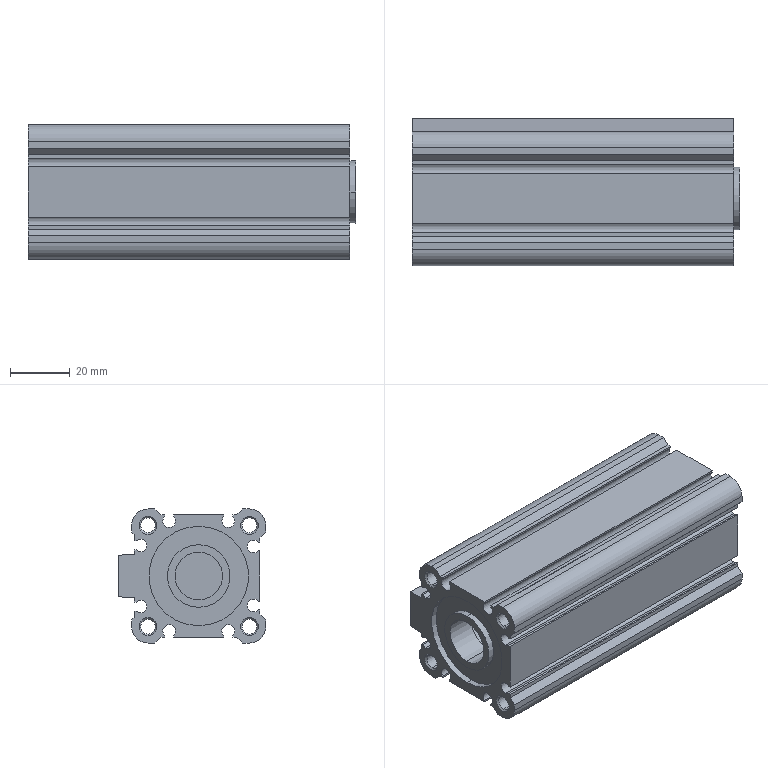Part | SolidWorks | features BaseBody 1 | 1 solid | 145 faces | box 110 x 49.5 x 45 mm | volume 111892 mm3 | plane 65 | cylinder 60 | cone 20 | commonest cylinder face diameters 4.26 x18 4.917 x16 6 x8 8.566 x4 11 x4 21 x4